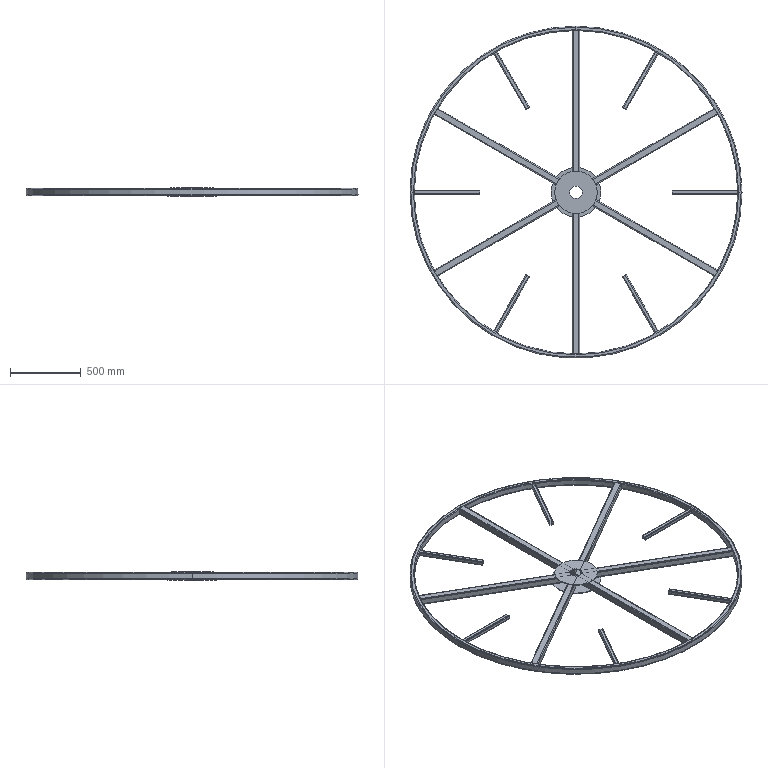Part | SolidWorks | features WeldMemberFeat 3, ICE 2, 3DProfileFeature 1, Cut 1, WeldmentFeature 1 | 15 solids | 292 faces | box 2340 x 2340 x 60 mm | volume 8212314 mm3 | plane 126 | cylinder 112 | torus 30 | cone 24 | commonest cylinder face diameters 12 x56 6 x48 87.5 x4 300 x2 350 x2